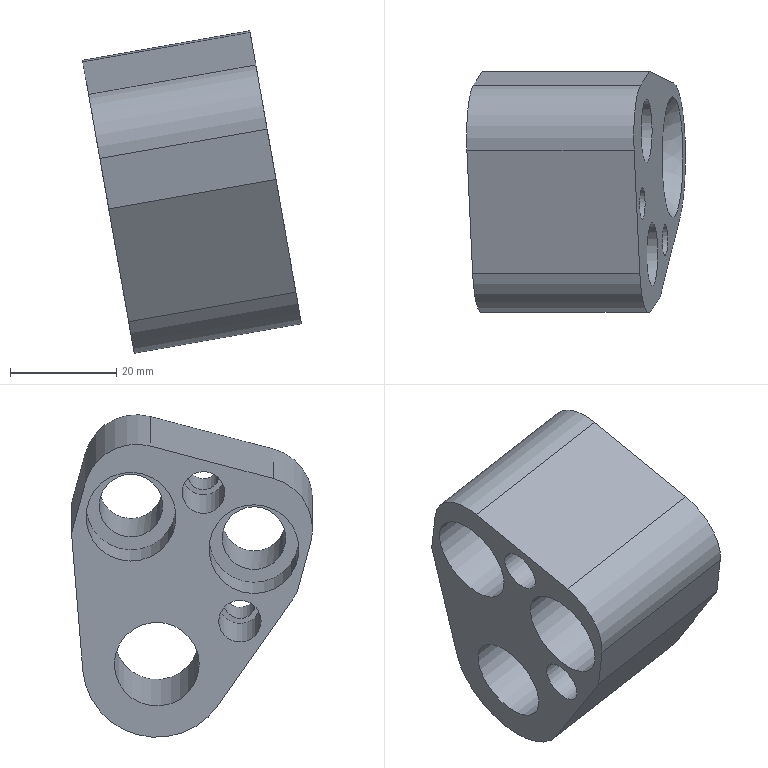Part | NX | features solid 2 | 1 solid | 24 faces | box 41.253 x 45.43 x 60.788 mm | volume 40894 mm3 | cylinder 12 | plane 11 | cone 1 | commonest cylinder face diameters 6 x2 8 x2 12 x2 17 x2 20 x2 16 x1
STEP:
#1=CARTESIAN_POINT('',(-508.615,-60.243,68.026));
#2=VERTEX_POINT('',#1);
#3=CARTESIAN_POINT('',(-508.795,-56.379,69.046));
#4=DIRECTION('',(-0.9848,0.,-0.1736));
#5=DIRECTION('',(0.04494,-0.9659,-0.2549));
#6=AXIS2_PLACEMENT_3D('',#3,#4,#5);
#7=CIRCLE('',#6,4.);
#8=EDGE_CURVE('',#2,#2,#7,.F.);
#9=ORIENTED_EDGE('',*,*,#8,.T.);
#10=EDGE_LOOP('',(#9));
#11=FACE_BOUND('',#10,.T.);
#12=CARTESIAN_POINT('',(-509.418,-44.918,72.58));
#13=VERTEX_POINT('',#12);
#14=CARTESIAN_POINT('',(-507.992,-42.718,64.494));
#15=DIRECTION('',(0.9848,0.,0.1736));
#16=DIRECTION('',(-0.1677,-0.2588,0.9513));
#17=AXIS2_PLACEMENT_3D('',#14,#15,#16);
#18=CIRCLE('',#17,8.5);
#19=EDGE_CURVE('',#13,#13,#18,.T.);
#20=ORIENTED_EDGE('',*,*,#19,.T.);
#21=EDGE_LOOP('',(#20));
#22=FACE_BOUND('',#21,.T.);
#23=CARTESIAN_POINT('',(-508.339,-68.1,66.463));
#24=VERTEX_POINT('',#23);
#25=CARTESIAN_POINT('',(-506.914,-65.9,58.377));
#26=DIRECTION('',(0.9848,0.,0.1736));
#27=DIRECTION('',(-0.1677,-0.2588,0.9513));
#28=AXIS2_PLACEMENT_3D('',#25,#26,#27);
#29=CIRCLE('',#28,8.5);
#30=EDGE_CURVE('',#24,#24,#29,.T.);
#31=ORIENTED_EDGE('',*,*,#30,.T.);
#32=EDGE_LOOP('',(#31));
#33=FACE_BOUND('',#32,.T.);
#34=CARTESIAN_POINT('',(-502.732,-55.307,34.664));
#35=VERTEX_POINT('',#34);
#36=CARTESIAN_POINT('',(-503.092,-47.58,36.703));
#37=DIRECTION('',(-0.9848,0.,-0.1736));
#38=DIRECTION('',(0.04494,-0.9659,-0.2549));
#39=AXIS2_PLACEMENT_3D('',#36,#37,#38);
#40=CIRCLE('',#39,8.);
#41=EDGE_CURVE('',#35,#35,#40,.T.);
#42=ORIENTED_EDGE('',*,*,#41,.F.);
#43=EDGE_LOOP('',(#42));
#44=FACE_BOUND('',#43,.T.);
#45=CARTESIAN_POINT('',(-509.113,-34.094,70.848));
#46=VERTEX_POINT('',#45);
#47=CARTESIAN_POINT('',(-510.34,-46.341,77.812));
#48=VERTEX_POINT('',#47);
#49=CARTESIAN_POINT('',(-508.663,-43.753,68.299));
#50=DIRECTION('',(0.9848,0.,0.1736));
#51=DIRECTION('',(-0.1677,-0.2588,0.9513));
#52=AXIS2_PLACEMENT_3D('',#49,#50,#51);
#53=CIRCLE('',#52,10.);
#54=EDGE_CURVE('',#46,#48,#53,.T.);
#55=ORIENTED_EDGE('',*,*,#54,.F.);
#56=CARTESIAN_POINT('',(-507.435,-31.506,61.336));
#57=VERTEX_POINT('',#56);
#58=CARTESIAN_POINT('',(-507.435,-31.506,61.336));
#59=DIRECTION('',(-0.1677,-0.2588,0.9513));
#60=VECTOR('',#59,1000.);
#61=LINE('',#58,#60);
#62=EDGE_CURVE('',#57,#46,#61,.T.);
#63=ORIENTED_EDGE('',*,*,#62,.F.);
#64=CARTESIAN_POINT('',(-502.895,-33.625,35.589));
#65=VERTEX_POINT('',#64);
#66=CARTESIAN_POINT('',(-502.895,-33.625,35.589));
#67=DIRECTION('',(-0.1731,0.08082,0.9816));
#68=VECTOR('',#67,1000.);
#69=LINE('',#66,#68);
#70=EDGE_CURVE('',#65,#57,#69,.T.);
#71=ORIENTED_EDGE('',*,*,#70,.F.);
#72=CARTESIAN_POINT('',(-501.71,-59.099,28.867));
#73=VERTEX_POINT('',#72);
#74=CARTESIAN_POINT('',(-503.092,-47.58,36.703));
#75=DIRECTION('',(0.9848,0.,0.1736));
#76=DIRECTION('',(-0.1677,-0.2588,0.9513));
#77=AXIS2_PLACEMENT_3D('',#74,#75,#76);
#78=CIRCLE('',#77,14.);
#79=EDGE_CURVE('',#73,#65,#78,.T.);
#80=ORIENTED_EDGE('',*,*,#79,.F.);
#81=CARTESIAN_POINT('',(-505.458,-74.006,50.121));
#82=VERTEX_POINT('',#81);
#83=CARTESIAN_POINT('',(-501.71,-59.099,28.867));
#84=DIRECTION('',(-0.1429,-0.5684,0.8103));
#85=VECTOR('',#84,1000.);
#86=LINE('',#83,#85);
#87=EDGE_CURVE('',#73,#82,#86,.T.);
#88=ORIENTED_EDGE('',*,*,#87,.T.);
#89=CARTESIAN_POINT('',(-507.135,-76.594,59.633));
#90=VERTEX_POINT('',#89);
#91=CARTESIAN_POINT('',(-505.458,-74.006,50.121));
#92=DIRECTION('',(-0.1677,-0.2588,0.9513));
#93=VECTOR('',#92,1000.);
#94=LINE('',#91,#93);
#95=EDGE_CURVE('',#82,#90,#94,.T.);
#96=ORIENTED_EDGE('',*,*,#95,.T.);
#97=CARTESIAN_POINT('',(-509.262,-69.523,71.695));
#98=VERTEX_POINT('',#97);
#99=CARTESIAN_POINT('',(-507.584,-66.935,62.182));
#100=DIRECTION('',(0.9848,0.,0.1736));
#101=DIRECTION('',(-0.1677,-0.2588,0.9513));
#102=AXIS2_PLACEMENT_3D('',#99,#100,#101);
#103=CIRCLE('',#102,10.);
#104=EDGE_CURVE('',#98,#90,#103,.T.);
#105=ORIENTED_EDGE('',*,*,#104,.F.);
#106=CARTESIAN_POINT('',(-509.262,-69.523,71.695));
#107=DIRECTION('',(-0.04494,0.9659,0.2549));
#108=VECTOR('',#107,1000.);
#109=LINE('',#106,#108);
#110=EDGE_CURVE('',#98,#48,#109,.T.);
#111=ORIENTED_EDGE('',*,*,#110,.T.);
#112=EDGE_LOOP('',(#55,#63,#71,#80,#88,#96,#105,#111));
#113=FACE_BOUND('',#112,.T.);
#114=CARTESIAN_POINT('',(-504.341,-67.106,43.785));
#115=VERTEX_POINT('',#114);
#116=CARTESIAN_POINT('',(-504.52,-63.242,44.805));
#117=DIRECTION('',(-0.9848,0.,-0.1736));
#118=DIRECTION('',(0.04494,-0.9659,-0.2549));
#119=AXIS2_PLACEMENT_3D('',#116,#117,#118);
#120=CIRCLE('',#119,4.);
#121=EDGE_CURVE('',#115,#115,#120,.F.);
#122=ORIENTED_EDGE('',*,*,#121,.T.);
#123=EDGE_LOOP('',(#122));
#124=FACE_BOUND('',#123,.T.);
#125=CARTESIAN_POINT('',(-508.663,-43.753,68.299));
#126=DIRECTION('',(-0.9848,0.,-0.1736));
#127=DIRECTION('',(-0.04494,0.9659,0.2549));
#128=AXIS2_PLACEMENT_3D('',#125,#126,#127);
#129=PLANE('',#128);
#130=ADVANCED_FACE('',(#11,#22,#33,#44,#113,#124),#129,.T.);
#131=CARTESIAN_POINT('',(-477.485,-44.271,75.759));
#132=VERTEX_POINT('',#131);
#133=CARTESIAN_POINT('',(-476.478,-42.718,70.051));
#134=DIRECTION('',(0.9848,0.,0.1736));
#135=DIRECTION('',(-0.1677,-0.2588,0.9513));
#136=AXIS2_PLACEMENT_3D('',#133,#134,#135);
#137=CIRCLE('',#136,6.);
#138=EDGE_CURVE('',#132,#132,#137,.T.);
#139=ORIENTED_EDGE('',*,*,#138,.T.);
#140=EDGE_LOOP('',(#139));
#141=FACE_BOUND('',#140,.T.);
#142=CARTESIAN_POINT('',(-496.444,-36.922,68.107));
#143=VERTEX_POINT('',#142);
#144=CARTESIAN_POINT('',(-496.174,-42.718,66.578));
#145=DIRECTION('',(0.9848,0.,0.1736));
#146=DIRECTION('',(-0.04494,0.9659,0.2549));
#147=AXIS2_PLACEMENT_3D('',#144,#145,#146);
#148=CIRCLE('',#147,6.);
#149=EDGE_CURVE('',#143,#143,#148,.T.);
#150=ORIENTED_EDGE('',*,*,#149,.F.);
#151=EDGE_LOOP('',(#150));
#152=FACE_BOUND('',#151,.T.);
#153=CARTESIAN_POINT('',(-507.992,-42.718,64.494));
#154=DIRECTION('',(0.9848,0.,0.1736));
#155=DIRECTION('',(0.04494,-0.9659,-0.2549));
#156=AXIS2_PLACEMENT_3D('',#153,#154,#155);
#157=CYLINDRICAL_SURFACE('',#156,6.);
#158=ADVANCED_FACE('',(#141,#152),#157,.F.);
#159=CARTESIAN_POINT('',(-476.406,-67.453,69.641));
#160=VERTEX_POINT('',#159);
#161=CARTESIAN_POINT('',(-475.4,-65.9,63.934));
#162=DIRECTION('',(0.9848,0.,0.1736));
#163=DIRECTION('',(-0.1677,-0.2588,0.9513));
#164=AXIS2_PLACEMENT_3D('',#161,#162,#163);
#165=CIRCLE('',#164,6.);
#166=EDGE_CURVE('',#160,#160,#165,.T.);
#167=ORIENTED_EDGE('',*,*,#166,.T.);
#168=EDGE_LOOP('',(#167));
#169=FACE_BOUND('',#168,.T.);
#170=CARTESIAN_POINT('',(-495.365,-60.104,61.99));
#171=VERTEX_POINT('',#170);
#172=CARTESIAN_POINT('',(-495.096,-65.9,60.461));
#173=DIRECTION('',(0.9848,0.,0.1736));
#174=DIRECTION('',(-0.04494,0.9659,0.2549));
#175=AXIS2_PLACEMENT_3D('',#172,#173,#174);
#176=CIRCLE('',#175,6.);
#177=EDGE_CURVE('',#171,#171,#176,.T.);
#178=ORIENTED_EDGE('',*,*,#177,.F.);
#179=EDGE_LOOP('',(#178));
#180=FACE_BOUND('',#179,.T.);
#181=CARTESIAN_POINT('',(-506.914,-65.9,58.377));
#182=DIRECTION('',(0.9848,0.,0.1736));
#183=DIRECTION('',(0.04494,-0.9659,-0.2549));
#184=AXIS2_PLACEMENT_3D('',#181,#182,#183);
#185=CYLINDRICAL_SURFACE('',#184,6.);
#186=ADVANCED_FACE('',(#169,#180),#185,.F.);
#187=CARTESIAN_POINT('',(-473.51,-64.019,53.215));
#188=VERTEX_POINT('',#187);
#189=CARTESIAN_POINT('',(-473.006,-63.242,50.361));
#190=DIRECTION('',(0.9848,0.,0.1736));
#191=DIRECTION('',(-0.1677,-0.2588,0.9513));
#192=AXIS2_PLACEMENT_3D('',#189,#190,#191);
#193=CIRCLE('',#192,3.);
#194=EDGE_CURVE('',#188,#188,#193,.T.);
#195=ORIENTED_EDGE('',*,*,#194,.F.);
#196=EDGE_LOOP('',(#195));
#197=FACE_BOUND('',#196,.T.);
#198=ORIENTED_EDGE('',*,*,#166,.F.);
#199=EDGE_LOOP('',(#198));
#200=FACE_BOUND('',#199,.T.);
#201=CARTESIAN_POINT('',(-472.09,-36.568,45.166));
#202=VERTEX_POINT('',#201);
#203=CARTESIAN_POINT('',(-471.578,-47.58,42.26));
#204=DIRECTION('',(0.9848,0.,0.1736));
#205=DIRECTION('',(-0.04494,0.9659,0.2549));
#206=AXIS2_PLACEMENT_3D('',#203,#204,#205);
#207=CIRCLE('',#206,11.4);
#208=EDGE_CURVE('',#202,#202,#207,.T.);
#209=ORIENTED_EDGE('',*,*,#208,.F.);
#210=EDGE_LOOP('',(#209));
#211=FACE_BOUND('',#210,.T.);
#212=CARTESIAN_POINT('',(-477.599,-34.094,76.405));
#213=VERTEX_POINT('',#212);
#214=CARTESIAN_POINT('',(-478.827,-46.341,83.369));
#215=VERTEX_POINT('',#214);
#216=CARTESIAN_POINT('',(-477.149,-43.753,73.856));
#217=DIRECTION('',(0.9848,0.,0.1736));
#218=DIRECTION('',(-0.1677,-0.2588,0.9513));
#219=AXIS2_PLACEMENT_3D('',#216,#217,#218);
#220=CIRCLE('',#219,10.);
#221=EDGE_CURVE('',#213,#215,#220,.T.);
#222=ORIENTED_EDGE('',*,*,#221,.T.);
#223=CARTESIAN_POINT('',(-477.748,-69.523,77.251));
#224=VERTEX_POINT('',#223);
#225=CARTESIAN_POINT('',(-477.748,-69.523,77.251));
#226=DIRECTION('',(-0.04494,0.9659,0.2549));
#227=VECTOR('',#226,1000.);
#228=LINE('',#225,#227);
#229=EDGE_CURVE('',#224,#215,#228,.T.);
#230=ORIENTED_EDGE('',*,*,#229,.F.);
#231=CARTESIAN_POINT('',(-475.621,-76.594,65.19));
#232=VERTEX_POINT('',#231);
#233=CARTESIAN_POINT('',(-476.071,-66.935,67.739));
#234=DIRECTION('',(0.9848,0.,0.1736));
#235=DIRECTION('',(-0.1677,-0.2588,0.9513));
#236=AXIS2_PLACEMENT_3D('',#233,#234,#235);
#237=CIRCLE('',#236,10.);
#238=EDGE_CURVE('',#224,#232,#237,.T.);
#239=ORIENTED_EDGE('',*,*,#238,.T.);
#240=CARTESIAN_POINT('',(-473.944,-74.006,55.677));
#241=VERTEX_POINT('',#240);
#242=CARTESIAN_POINT('',(-473.944,-74.006,55.677));
#243=DIRECTION('',(-0.1677,-0.2588,0.9513));
#244=VECTOR('',#243,1000.);
#245=LINE('',#242,#244);
#246=EDGE_CURVE('',#241,#232,#245,.T.);
#247=ORIENTED_EDGE('',*,*,#246,.F.);
#248=CARTESIAN_POINT('',(-470.196,-59.099,34.424));
#249=VERTEX_POINT('',#248);
#250=CARTESIAN_POINT('',(-470.196,-59.099,34.424));
#251=DIRECTION('',(-0.1429,-0.5684,0.8103));
#252=VECTOR('',#251,1000.);
#253=LINE('',#250,#252);
#254=EDGE_CURVE('',#249,#241,#253,.T.);
#255=ORIENTED_EDGE('',*,*,#254,.F.);
#256=CARTESIAN_POINT('',(-471.381,-33.625,41.146));
#257=VERTEX_POINT('',#256);
#258=CARTESIAN_POINT('',(-471.578,-47.58,42.26));
#259=DIRECTION('',(0.9848,0.,0.1736));
#260=DIRECTION('',(-0.1677,-0.2588,0.9513));
#261=AXIS2_PLACEMENT_3D('',#258,#259,#260);
#262=CIRCLE('',#261,14.);
#263=EDGE_CURVE('',#249,#257,#262,.T.);
#264=ORIENTED_EDGE('',*,*,#263,.T.);
#265=CARTESIAN_POINT('',(-475.921,-31.506,66.892));
#266=VERTEX_POINT('',#265);
#267=CARTESIAN_POINT('',(-471.381,-33.625,41.146));
#268=DIRECTION('',(-0.1731,0.08082,0.9816));
#269=VECTOR('',#268,1000.);
#270=LINE('',#267,#269);
#271=EDGE_CURVE('',#257,#266,#270,.T.);
#272=ORIENTED_EDGE('',*,*,#271,.T.);
#273=CARTESIAN_POINT('',(-475.921,-31.506,66.892));
#274=DIRECTION('',(-0.1677,-0.2588,0.9513));
#275=VECTOR('',#274,1000.);
#276=LINE('',#273,#275);
#277=EDGE_CURVE('',#266,#213,#276,.T.);
#278=ORIENTED_EDGE('',*,*,#277,.T.);
#279=EDGE_LOOP('',(#222,#230,#239,#247,#255,#264,#272,#278));
#280=FACE_BOUND('',#279,.T.);
#281=ORIENTED_EDGE('',*,*,#138,.F.);
#282=EDGE_LOOP('',(#281));
#283=FACE_BOUND('',#282,.T.);
#284=CARTESIAN_POINT('',(-477.784,-57.156,77.456));
#285=VERTEX_POINT('',#284);
#286=CARTESIAN_POINT('',(-477.281,-56.379,74.603));
#287=DIRECTION('',(0.9848,0.,0.1736));
#288=DIRECTION('',(-0.1677,-0.2588,0.9513));
#289=AXIS2_PLACEMENT_3D('',#286,#287,#288);
#290=CIRCLE('',#289,3.);
#291=EDGE_CURVE('',#285,#285,#290,.T.);
#292=ORIENTED_EDGE('',*,*,#291,.F.);
#293=EDGE_LOOP('',(#292));
#294=FACE_BOUND('',#293,.T.);
#295=CARTESIAN_POINT('',(-477.149,-43.753,73.856));
#296=DIRECTION('',(-0.9848,0.,-0.1736));
#297=DIRECTION('',(-0.04494,0.9659,0.2549));
#298=AXIS2_PLACEMENT_3D('',#295,#296,#297);
#299=PLANE('',#298);
#300=ADVANCED_FACE('',(#197,#200,#211,#280,#283,#294),#299,.F.);
#301=ORIENTED_EDGE('',*,*,#221,.F.);
#302=CARTESIAN_POINT('',(-509.113,-34.094,70.848));
#303=DIRECTION('',(0.9848,0.,0.1736));
#304=VECTOR('',#303,1000.);
#305=LINE('',#302,#304);
#306=EDGE_CURVE('',#46,#213,#305,.T.);
#307=ORIENTED_EDGE('',*,*,#306,.F.);
#308=ORIENTED_EDGE('',*,*,#54,.T.);
#309=CARTESIAN_POINT('',(-510.34,-46.341,77.812));
#310=DIRECTION('',(0.9848,0.,0.1736));
#311=VECTOR('',#310,1000.);
#312=LINE('',#309,#311);
#313=EDGE_CURVE('',#48,#215,#312,.T.);
#314=ORIENTED_EDGE('',*,*,#313,.T.);
#315=EDGE_LOOP('',(#301,#307,#308,#314));
#316=FACE_BOUND('',#315,.T.);
#317=CARTESIAN_POINT('',(-508.663,-43.753,68.299));
#318=DIRECTION('',(0.9848,0.,0.1736));
#319=DIRECTION('',(0.04494,-0.9659,-0.2549));
#320=AXIS2_PLACEMENT_3D('',#317,#318,#319);
#321=CYLINDRICAL_SURFACE('',#320,10.);
#322=ADVANCED_FACE('',(#316),#321,.T.);
#323=ORIENTED_EDGE('',*,*,#229,.T.);
#324=ORIENTED_EDGE('',*,*,#313,.F.);
#325=ORIENTED_EDGE('',*,*,#110,.F.);
#326=CARTESIAN_POINT('',(-509.262,-69.523,71.695));
#327=DIRECTION('',(0.9848,0.,0.1736));
#328=VECTOR('',#327,1000.);
#329=LINE('',#326,#328);
#330=EDGE_CURVE('',#98,#224,#329,.T.);
#331=ORIENTED_EDGE('',*,*,#330,.T.);
#332=EDGE_LOOP('',(#323,#324,#325,#331));
#333=FACE_BOUND('',#332,.T.);
#334=CARTESIAN_POINT('',(-509.262,-69.523,71.695));
#335=DIRECTION('',(-0.1677,-0.2588,0.9513));
#336=DIRECTION('',(-0.04494,0.9659,0.2549));
#337=AXIS2_PLACEMENT_3D('',#334,#335,#336);
#338=PLANE('',#337);
#339=ADVANCED_FACE('',(#333),#338,.T.);
#340=ORIENTED_EDGE('',*,*,#238,.F.);
#341=ORIENTED_EDGE('',*,*,#330,.F.);
#342=ORIENTED_EDGE('',*,*,#104,.T.);
#343=CARTESIAN_POINT('',(-507.135,-76.594,59.633));
#344=DIRECTION('',(0.9848,0.,0.1736));
#345=VECTOR('',#344,1000.);
#346=LINE('',#343,#345);
#347=EDGE_CURVE('',#90,#232,#346,.T.);
#348=ORIENTED_EDGE('',*,*,#347,.T.);
#349=EDGE_LOOP('',(#340,#341,#342,#348));
#350=FACE_BOUND('',#349,.T.);
#351=CARTESIAN_POINT('',(-507.584,-66.935,62.182));
#352=DIRECTION('',(0.9848,0.,0.1736));
#353=DIRECTION('',(0.04494,-0.9659,-0.2549));
#354=AXIS2_PLACEMENT_3D('',#351,#352,#353);
#355=CYLINDRICAL_SURFACE('',#354,10.);
#356=ADVANCED_FACE('',(#350),#355,.T.);
#357=ORIENTED_EDGE('',*,*,#246,.T.);
#358=ORIENTED_EDGE('',*,*,#347,.F.);
#359=ORIENTED_EDGE('',*,*,#95,.F.);
#360=CARTESIAN_POINT('',(-505.458,-74.006,50.121));
#361=DIRECTION('',(0.9848,0.,0.1736));
#362=VECTOR('',#361,1000.);
#363=LINE('',#360,#362);
#364=EDGE_CURVE('',#82,#241,#363,.T.);
#365=ORIENTED_EDGE('',*,*,#364,.T.);
#366=EDGE_LOOP('',(#357,#358,#359,#365));
#367=FACE_BOUND('',#366,.T.);
#368=CARTESIAN_POINT('',(-505.458,-74.006,50.121));
#369=DIRECTION('',(0.04494,-0.9659,-0.2549));
#370=DIRECTION('',(-0.9848,0.,-0.1736));
#371=AXIS2_PLACEMENT_3D('',#368,#369,#370);
#372=PLANE('',#371);
#373=ADVANCED_FACE('',(#367),#372,.T.);
#374=ORIENTED_EDGE('',*,*,#254,.T.);
#375=ORIENTED_EDGE('',*,*,#364,.F.);
#376=ORIENTED_EDGE('',*,*,#87,.F.);
#377=CARTESIAN_POINT('',(-501.71,-59.099,28.867));
#378=DIRECTION('',(0.9848,0.,0.1736));
#379=VECTOR('',#378,1000.);
#380=LINE('',#377,#379);
#381=EDGE_CURVE('',#73,#249,#380,.T.);
#382=ORIENTED_EDGE('',*,*,#381,.T.);
#383=EDGE_LOOP('',(#374,#375,#376,#382));
#384=FACE_BOUND('',#383,.T.);
#385=CARTESIAN_POINT('',(-501.71,-59.099,28.867));
#386=DIRECTION('',(0.09869,-0.8228,-0.5597));
#387=DIRECTION('',(-0.1429,-0.5684,0.8103));
#388=AXIS2_PLACEMENT_3D('',#385,#386,#387);
#389=PLANE('',#388);
#390=ADVANCED_FACE('',(#384),#389,.T.);
#391=ORIENTED_EDGE('',*,*,#263,.F.);
#392=ORIENTED_EDGE('',*,*,#381,.F.);
#393=ORIENTED_EDGE('',*,*,#79,.T.);
#394=CARTESIAN_POINT('',(-502.895,-33.625,35.589));
#395=DIRECTION('',(0.9848,0.,0.1736));
#396=VECTOR('',#395,1000.);
#397=LINE('',#394,#396);
#398=EDGE_CURVE('',#65,#257,#397,.T.);
#399=ORIENTED_EDGE('',*,*,#398,.T.);
#400=EDGE_LOOP('',(#391,#392,#393,#399));
#401=FACE_BOUND('',#400,.T.);
#402=CARTESIAN_POINT('',(-503.092,-47.58,36.703));
#403=DIRECTION('',(0.9848,0.,0.1736));
#404=DIRECTION('',(0.04494,-0.9659,-0.2549));
#405=AXIS2_PLACEMENT_3D('',#402,#403,#404);
#406=CYLINDRICAL_SURFACE('',#405,14.);
#407=ADVANCED_FACE('',(#401),#406,.T.);
#408=ORIENTED_EDGE('',*,*,#271,.F.);
#409=ORIENTED_EDGE('',*,*,#398,.F.);
#410=ORIENTED_EDGE('',*,*,#70,.T.);
#411=CARTESIAN_POINT('',(-507.435,-31.506,61.336));
#412=DIRECTION('',(0.9848,0.,0.1736));
#413=VECTOR('',#412,1000.);
#414=LINE('',#411,#413);
#415=EDGE_CURVE('',#57,#266,#414,.T.);
#416=ORIENTED_EDGE('',*,*,#415,.T.);
#417=EDGE_LOOP('',(#408,#409,#410,#416));
#418=FACE_BOUND('',#417,.T.);
#419=CARTESIAN_POINT('',(-502.895,-33.625,35.589));
#420=DIRECTION('',(-0.01403,-0.9967,0.07959));
#421=DIRECTION('',(-0.1731,0.08082,0.9816));
#422=AXIS2_PLACEMENT_3D('',#419,#420,#421);
#423=PLANE('',#422);
#424=ADVANCED_FACE('',(#418),#423,.F.);
#425=ORIENTED_EDGE('',*,*,#277,.F.);
#426=ORIENTED_EDGE('',*,*,#415,.F.);
#427=ORIENTED_EDGE('',*,*,#62,.T.);
#428=ORIENTED_EDGE('',*,*,#306,.T.);
#429=EDGE_LOOP('',(#425,#426,#427,#428));
#430=FACE_BOUND('',#429,.T.);
#431=CARTESIAN_POINT('',(-507.435,-31.506,61.336));
#432=DIRECTION('',(0.04494,-0.9659,-0.2549));
#433=DIRECTION('',(-0.1677,-0.2588,0.9513));
#434=AXIS2_PLACEMENT_3D('',#431,#432,#433);
#435=PLANE('',#434);
#436=ADVANCED_FACE('',(#430),#435,.F.);
#437=ORIENTED_EDGE('',*,*,#41,.T.);
#438=EDGE_LOOP('',(#437));
#439=FACE_BOUND('',#438,.T.);
#440=CARTESIAN_POINT('',(-474.567,-55.307,39.63));
#441=VERTEX_POINT('',#440);
#442=CARTESIAN_POINT('',(-474.926,-47.58,41.67));
#443=DIRECTION('',(0.9848,0.,0.1736));
#444=DIRECTION('',(0.04494,-0.9659,-0.2549));
#445=AXIS2_PLACEMENT_3D('',#442,#443,#444);
#446=CIRCLE('',#445,8.);
#447=EDGE_CURVE('',#441,#441,#446,.T.);
#448=ORIENTED_EDGE('',*,*,#447,.T.);
#449=EDGE_LOOP('',(#448));
#450=FACE_BOUND('',#449,.T.);
#451=CARTESIAN_POINT('',(-503.092,-47.58,36.703));
#452=DIRECTION('',(0.9848,0.,0.1736));
#453=DIRECTION('',(0.04494,-0.9659,-0.2549));
#454=AXIS2_PLACEMENT_3D('',#451,#452,#453);
#455=CYLINDRICAL_SURFACE('',#454,8.);
#456=ADVANCED_FACE('',(#439,#450),#455,.F.);
#457=ORIENTED_EDGE('',*,*,#208,.T.);
#458=EDGE_LOOP('',(#457));
#459=FACE_BOUND('',#458,.T.);
#460=ORIENTED_EDGE('',*,*,#447,.F.);
#461=EDGE_LOOP('',(#460));
#462=FACE_BOUND('',#461,.T.);
#463=CARTESIAN_POINT('',(-474.926,-47.58,41.67));
#464=DIRECTION('',(0.9848,0.,0.1736));
#465=DIRECTION('',(0.04494,-0.9659,-0.2549));
#466=AXIS2_PLACEMENT_3D('',#463,#464,#465);
#467=CONICAL_SURFACE('',#466,8.,0.7854);
#468=ADVANCED_FACE('',(#459,#462),#467,.F.);
#469=CARTESIAN_POINT('',(-485.327,-64.019,51.131));
#470=VERTEX_POINT('',#469);
#471=CARTESIAN_POINT('',(-484.824,-63.242,48.278));
#472=DIRECTION('',(0.9848,0.,0.1736));
#473=DIRECTION('',(-0.1677,-0.2588,0.9513));
#474=AXIS2_PLACEMENT_3D('',#471,#472,#473);
#475=CIRCLE('',#474,3.);
#476=EDGE_CURVE('',#470,#470,#475,.T.);
#477=ORIENTED_EDGE('',*,*,#476,.F.);
#478=EDGE_LOOP('',(#477));
#479=FACE_BOUND('',#478,.T.);
#480=ORIENTED_EDGE('',*,*,#194,.T.);
#481=EDGE_LOOP('',(#480));
#482=FACE_BOUND('',#481,.T.);
#483=CARTESIAN_POINT('',(-504.52,-63.242,44.805));
#484=DIRECTION('',(0.9848,0.,0.1736));
#485=DIRECTION('',(0.04494,-0.9659,-0.2549));
#486=AXIS2_PLACEMENT_3D('',#483,#484,#485);
#487=CYLINDRICAL_SURFACE('',#486,3.);
#488=ADVANCED_FACE('',(#479,#482),#487,.F.);
#489=CARTESIAN_POINT('',(-489.602,-57.156,75.372));
#490=VERTEX_POINT('',#489);
#491=CARTESIAN_POINT('',(-489.099,-56.379,72.519));
#492=DIRECTION('',(0.9848,0.,0.1736));
#493=DIRECTION('',(-0.1677,-0.2588,0.9513));
#494=AXIS2_PLACEMENT_3D('',#491,#492,#493);
#495=CIRCLE('',#494,3.);
#496=EDGE_CURVE('',#490,#490,#495,.T.);
#497=ORIENTED_EDGE('',*,*,#496,.F.);
#498=EDGE_LOOP('',(#497));
#499=FACE_BOUND('',#498,.T.);
#500=ORIENTED_EDGE('',*,*,#291,.T.);
#501=EDGE_LOOP('',(#500));
#502=FACE_BOUND('',#501,.T.);
#503=CARTESIAN_POINT('',(-508.795,-56.379,69.046));
#504=DIRECTION('',(0.9848,0.,0.1736));
#505=DIRECTION('',(0.04494,-0.9659,-0.2549));
#506=AXIS2_PLACEMENT_3D('',#503,#504,#505);
#507=CYLINDRICAL_SURFACE('',#506,3.);
#508=ADVANCED_FACE('',(#499,#502),#507,.F.);
#509=CARTESIAN_POINT('',(-496.522,-68.1,68.547));
#510=VERTEX_POINT('',#509);
#511=CARTESIAN_POINT('',(-495.096,-65.9,60.461));
#512=DIRECTION('',(0.9848,0.,0.1736));
#513=DIRECTION('',(-0.1677,-0.2588,0.9513));
#514=AXIS2_PLACEMENT_3D('',#511,#512,#513);
#515=CIRCLE('',#514,8.5);
#516=EDGE_CURVE('',#510,#510,#515,.T.);
#517=ORIENTED_EDGE('',*,*,#516,.T.);
#518=EDGE_LOOP('',(#517));
#519=FACE_BOUND('',#518,.T.);
#520=ORIENTED_EDGE('',*,*,#30,.F.);
#521=EDGE_LOOP('',(#520));
#522=FACE_BOUND('',#521,.T.);
#523=CARTESIAN_POINT('',(-495.096,-65.9,60.461));
#524=DIRECTION('',(-0.9848,0.,-0.1736));
#525=DIRECTION('',(-0.04494,0.9659,0.2549));
#526=AXIS2_PLACEMENT_3D('',#523,#524,#525);
#527=CYLINDRICAL_SURFACE('',#526,8.5);
#528=ADVANCED_FACE('',(#519,#522),#527,.F.);
#529=ORIENTED_EDGE('',*,*,#177,.T.);
#530=EDGE_LOOP('',(#529));
#531=FACE_BOUND('',#530,.T.);
#532=ORIENTED_EDGE('',*,*,#516,.F.);
#533=EDGE_LOOP('',(#532));
#534=FACE_BOUND('',#533,.T.);
#535=CARTESIAN_POINT('',(-495.096,-65.9,60.461));
#536=DIRECTION('',(-0.9848,0.,-0.1736));
#537=DIRECTION('',(-0.04494,0.9659,0.2549));
#538=AXIS2_PLACEMENT_3D('',#535,#536,#537);
#539=PLANE('',#538);
#540=ADVANCED_FACE('',(#531,#534),#539,.T.);
#541=CARTESIAN_POINT('',(-497.6,-44.918,74.664));
#542=VERTEX_POINT('',#541);
#543=CARTESIAN_POINT('',(-496.174,-42.718,66.578));
#544=DIRECTION('',(0.9848,0.,0.1736));
#545=DIRECTION('',(-0.1677,-0.2588,0.9513));
#546=AXIS2_PLACEMENT_3D('',#543,#544,#545);
#547=CIRCLE('',#546,8.5);
#548=EDGE_CURVE('',#542,#542,#547,.T.);
#549=ORIENTED_EDGE('',*,*,#548,.T.);
#550=EDGE_LOOP('',(#549));
#551=FACE_BOUND('',#550,.T.);
#552=ORIENTED_EDGE('',*,*,#19,.F.);
#553=EDGE_LOOP('',(#552));
#554=FACE_BOUND('',#553,.T.);
#555=CARTESIAN_POINT('',(-496.174,-42.718,66.578));
#556=DIRECTION('',(-0.9848,0.,-0.1736));
#557=DIRECTION('',(-0.04494,0.9659,0.2549));
#558=AXIS2_PLACEMENT_3D('',#555,#556,#557);
#559=CYLINDRICAL_SURFACE('',#558,8.5);
#560=ADVANCED_FACE('',(#551,#554),#559,.F.);
#561=ORIENTED_EDGE('',*,*,#149,.T.);
#562=EDGE_LOOP('',(#561));
#563=FACE_BOUND('',#562,.T.);
#564=ORIENTED_EDGE('',*,*,#548,.F.);
#565=EDGE_LOOP('',(#564));
#566=FACE_BOUND('',#565,.T.);
#567=CARTESIAN_POINT('',(-496.174,-42.718,66.578));
#568=DIRECTION('',(-0.9848,0.,-0.1736));
#569=DIRECTION('',(-0.04494,0.9659,0.2549));
#570=AXIS2_PLACEMENT_3D('',#567,#568,#569);
#571=PLANE('',#570);
#572=ADVANCED_FACE('',(#563,#566),#571,.T.);
#573=CARTESIAN_POINT('',(-488.919,-60.243,71.499));
#574=VERTEX_POINT('',#573);
#575=CARTESIAN_POINT('',(-489.099,-56.379,72.519));
#576=DIRECTION('',(-0.9848,0.,-0.1736));
#577=DIRECTION('',(0.04494,-0.9659,-0.2549));
#578=AXIS2_PLACEMENT_3D('',#575,#576,#577);
#579=CIRCLE('',#578,4.);
#580=EDGE_CURVE('',#574,#574,#579,.F.);
#581=ORIENTED_EDGE('',*,*,#580,.F.);
#582=EDGE_LOOP('',(#581));
#583=FACE_BOUND('',#582,.T.);
#584=ORIENTED_EDGE('',*,*,#496,.T.);
#585=EDGE_LOOP('',(#584));
#586=FACE_BOUND('',#585,.T.);
#587=CARTESIAN_POINT('',(-489.099,-56.379,72.519));
#588=DIRECTION('',(0.9848,0.,0.1736));
#589=DIRECTION('',(0.04494,-0.9659,-0.2549));
#590=AXIS2_PLACEMENT_3D('',#587,#588,#589);
#591=PLANE('',#590);
#592=ADVANCED_FACE('',(#583,#586),#591,.F.);
#593=ORIENTED_EDGE('',*,*,#580,.T.);
#594=EDGE_LOOP('',(#593));
#595=FACE_BOUND('',#594,.T.);
#596=ORIENTED_EDGE('',*,*,#8,.F.);
#597=EDGE_LOOP('',(#596));
#598=FACE_BOUND('',#597,.T.);
#599=CARTESIAN_POINT('',(-508.795,-56.379,69.046));
#600=DIRECTION('',(0.9848,0.,0.1736));
#601=DIRECTION('',(0.04494,-0.9659,-0.2549));
#602=AXIS2_PLACEMENT_3D('',#599,#600,#601);
#603=CYLINDRICAL_SURFACE('',#602,4.);
#604=ADVANCED_FACE('',(#595,#598),#603,.F.);
#605=CARTESIAN_POINT('',(-484.644,-67.106,47.258));
#606=VERTEX_POINT('',#605);
#607=CARTESIAN_POINT('',(-484.824,-63.242,48.278));
#608=DIRECTION('',(-0.9848,0.,-0.1736));
#609=DIRECTION('',(0.04494,-0.9659,-0.2549));
#610=AXIS2_PLACEMENT_3D('',#607,#608,#609);
#611=CIRCLE('',#610,4.);
#612=EDGE_CURVE('',#606,#606,#611,.F.);
#613=ORIENTED_EDGE('',*,*,#612,.F.);
#614=EDGE_LOOP('',(#613));
#615=FACE_BOUND('',#614,.T.);
#616=ORIENTED_EDGE('',*,*,#476,.T.);
#617=EDGE_LOOP('',(#616));
#618=FACE_BOUND('',#617,.T.);
#619=CARTESIAN_POINT('',(-484.824,-63.242,48.278));
#620=DIRECTION('',(0.9848,0.,0.1736));
#621=DIRECTION('',(0.04494,-0.9659,-0.2549));
#622=AXIS2_PLACEMENT_3D('',#619,#620,#621);
#623=PLANE('',#622);
#624=ADVANCED_FACE('',(#615,#618),#623,.F.);
#625=ORIENTED_EDGE('',*,*,#612,.T.);
#626=EDGE_LOOP('',(#625));
#627=FACE_BOUND('',#626,.T.);
#628=ORIENTED_EDGE('',*,*,#121,.F.);
#629=EDGE_LOOP('',(#628));
#630=FACE_BOUND('',#629,.T.);
#631=CARTESIAN_POINT('',(-504.52,-63.242,44.805));
#632=DIRECTION('',(0.9848,0.,0.1736));
#633=DIRECTION('',(0.04494,-0.9659,-0.2549));
#634=AXIS2_PLACEMENT_3D('',#631,#632,#633);
#635=CYLINDRICAL_SURFACE('',#634,4.);
#636=ADVANCED_FACE('',(#627,#630),#635,.F.);
#637=CLOSED_SHELL('',(#130,#158,#186,#300,#322,#339,#356,#373,#390,#407,#424,#436,#456,#468,#488,#508,#528,#540,#560,#572,#592,#604,#624,#636));
#638=MANIFOLD_SOLID_BREP('',#637);
#639=(LENGTH_UNIT()NAMED_UNIT(*)SI_UNIT(.MILLI.,.METRE.));
#640=UNCERTAINTY_MEASURE_WITH_UNIT(LENGTH_MEASURE(0.00001),#639,'','');
#641=(NAMED_UNIT(*)PLANE_ANGLE_UNIT()SI_UNIT($,.RADIAN.));
#642=(NAMED_UNIT(*)SI_UNIT($,.STERADIAN.)SOLID_ANGLE_UNIT());
#643=(GEOMETRIC_REPRESENTATION_CONTEXT(3)GLOBAL_UNCERTAINTY_ASSIGNED_CONTEXT((#640))GLOBAL_UNIT_ASSIGNED_CONTEXT((#639,#641,#642))REPRESENTATION_CONTEXT('',''));
#644=ADVANCED_BREP_SHAPE_REPRESENTATION('',(#638),#643);